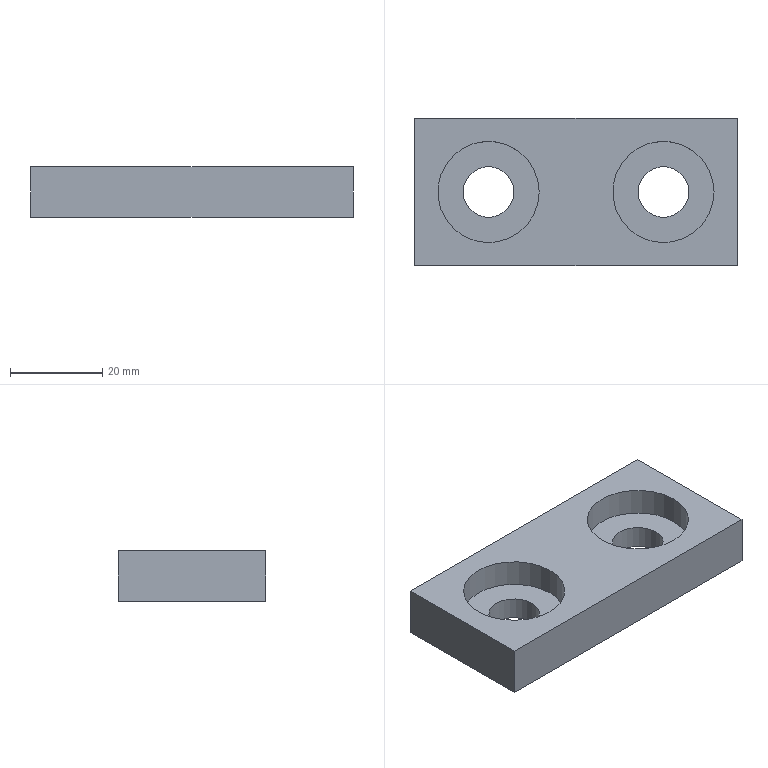Part | NX | features DATUM_CSYS 2, EXTRUDE 2, SKETCH 1 | 1 solid | 12 faces | box 70 x 32 x 11 mm | volume 19128 mm3 | plane 8 | cylinder 4 | commonest cylinder face diameters 11 x2 22 x2
STEP:
#1=CARTESIAN_POINT('',(-35.,16.,0.));
#2=VERTEX_POINT('',#1);
#3=CARTESIAN_POINT('',(-35.,-16.,0.));
#4=VERTEX_POINT('',#3);
#5=CARTESIAN_POINT('',(-35.,16.,0.));
#6=DIRECTION('',(0.,-1.,0.));
#7=VECTOR('',#6,1000.);
#8=LINE('',#5,#7);
#9=EDGE_CURVE('',#2,#4,#8,.T.);
#10=ORIENTED_EDGE('',*,*,#9,.T.);
#11=CARTESIAN_POINT('',(-35.,-16.,11.));
#12=VERTEX_POINT('',#11);
#13=CARTESIAN_POINT('',(-35.,-16.,11.));
#14=DIRECTION('',(0.,0.,-1.));
#15=VECTOR('',#14,1000.);
#16=LINE('',#13,#15);
#17=EDGE_CURVE('',#12,#4,#16,.T.);
#18=ORIENTED_EDGE('',*,*,#17,.F.);
#19=CARTESIAN_POINT('',(-35.,16.,11.));
#20=VERTEX_POINT('',#19);
#21=CARTESIAN_POINT('',(-35.,16.,11.));
#22=DIRECTION('',(0.,-1.,0.));
#23=VECTOR('',#22,1000.);
#24=LINE('',#21,#23);
#25=EDGE_CURVE('',#20,#12,#24,.T.);
#26=ORIENTED_EDGE('',*,*,#25,.F.);
#27=CARTESIAN_POINT('',(-35.,16.,11.));
#28=DIRECTION('',(0.,0.,-1.));
#29=VECTOR('',#28,1000.);
#30=LINE('',#27,#29);
#31=EDGE_CURVE('',#20,#2,#30,.T.);
#32=ORIENTED_EDGE('',*,*,#31,.T.);
#33=EDGE_LOOP('',(#10,#18,#26,#32));
#34=FACE_BOUND('',#33,.T.);
#35=CARTESIAN_POINT('',(-35.,16.,11.));
#36=DIRECTION('',(1.,0.,0.));
#37=DIRECTION('',(0.,0.,-1.));
#38=AXIS2_PLACEMENT_3D('',#35,#36,#37);
#39=PLANE('',#38);
#40=ADVANCED_FACE('',(#34),#39,.F.);
#41=CARTESIAN_POINT('',(35.,-16.,0.));
#42=VERTEX_POINT('',#41);
#43=CARTESIAN_POINT('',(-35.,-16.,0.));
#44=DIRECTION('',(1.,0.,0.));
#45=VECTOR('',#44,1000.);
#46=LINE('',#43,#45);
#47=EDGE_CURVE('',#4,#42,#46,.T.);
#48=ORIENTED_EDGE('',*,*,#47,.T.);
#49=CARTESIAN_POINT('',(35.,-16.,11.));
#50=VERTEX_POINT('',#49);
#51=CARTESIAN_POINT('',(35.,-16.,11.));
#52=DIRECTION('',(0.,0.,-1.));
#53=VECTOR('',#52,1000.);
#54=LINE('',#51,#53);
#55=EDGE_CURVE('',#50,#42,#54,.T.);
#56=ORIENTED_EDGE('',*,*,#55,.F.);
#57=CARTESIAN_POINT('',(-35.,-16.,11.));
#58=DIRECTION('',(1.,0.,0.));
#59=VECTOR('',#58,1000.);
#60=LINE('',#57,#59);
#61=EDGE_CURVE('',#12,#50,#60,.T.);
#62=ORIENTED_EDGE('',*,*,#61,.F.);
#63=ORIENTED_EDGE('',*,*,#17,.T.);
#64=EDGE_LOOP('',(#48,#56,#62,#63));
#65=FACE_BOUND('',#64,.T.);
#66=CARTESIAN_POINT('',(-35.,-16.,11.));
#67=DIRECTION('',(0.,1.,0.));
#68=DIRECTION('',(0.,0.,1.));
#69=AXIS2_PLACEMENT_3D('',#66,#67,#68);
#70=PLANE('',#69);
#71=ADVANCED_FACE('',(#65),#70,.F.);
#72=CARTESIAN_POINT('',(35.,16.,0.));
#73=VERTEX_POINT('',#72);
#74=CARTESIAN_POINT('',(35.,-16.,0.));
#75=DIRECTION('',(0.,1.,0.));
#76=VECTOR('',#75,1000.);
#77=LINE('',#74,#76);
#78=EDGE_CURVE('',#42,#73,#77,.T.);
#79=ORIENTED_EDGE('',*,*,#78,.T.);
#80=CARTESIAN_POINT('',(35.,16.,11.));
#81=VERTEX_POINT('',#80);
#82=CARTESIAN_POINT('',(35.,16.,11.));
#83=DIRECTION('',(0.,0.,-1.));
#84=VECTOR('',#83,1000.);
#85=LINE('',#82,#84);
#86=EDGE_CURVE('',#81,#73,#85,.T.);
#87=ORIENTED_EDGE('',*,*,#86,.F.);
#88=CARTESIAN_POINT('',(35.,-16.,11.));
#89=DIRECTION('',(0.,1.,0.));
#90=VECTOR('',#89,1000.);
#91=LINE('',#88,#90);
#92=EDGE_CURVE('',#50,#81,#91,.T.);
#93=ORIENTED_EDGE('',*,*,#92,.F.);
#94=ORIENTED_EDGE('',*,*,#55,.T.);
#95=EDGE_LOOP('',(#79,#87,#93,#94));
#96=FACE_BOUND('',#95,.T.);
#97=CARTESIAN_POINT('',(35.,-16.,11.));
#98=DIRECTION('',(-1.,0.,0.));
#99=DIRECTION('',(0.,0.,1.));
#100=AXIS2_PLACEMENT_3D('',#97,#98,#99);
#101=PLANE('',#100);
#102=ADVANCED_FACE('',(#96),#101,.F.);
#103=CARTESIAN_POINT('',(-8.,0.,5.));
#104=VERTEX_POINT('',#103);
#105=CARTESIAN_POINT('',(-19.,0.,5.));
#106=DIRECTION('',(0.,0.,1.));
#107=DIRECTION('',(1.,0.,0.));
#108=AXIS2_PLACEMENT_3D('',#105,#106,#107);
#109=CIRCLE('',#108,11.);
#110=EDGE_CURVE('',#104,#104,#109,.T.);
#111=ORIENTED_EDGE('',*,*,#110,.F.);
#112=EDGE_LOOP('',(#111));
#113=FACE_BOUND('',#112,.T.);
#114=CARTESIAN_POINT('',(-8.,0.,11.));
#115=VERTEX_POINT('',#114);
#116=CARTESIAN_POINT('',(-19.,0.,11.));
#117=DIRECTION('',(0.,0.,1.));
#118=DIRECTION('',(1.,0.,0.));
#119=AXIS2_PLACEMENT_3D('',#116,#117,#118);
#120=CIRCLE('',#119,11.);
#121=EDGE_CURVE('',#115,#115,#120,.T.);
#122=ORIENTED_EDGE('',*,*,#121,.T.);
#123=EDGE_LOOP('',(#122));
#124=FACE_BOUND('',#123,.T.);
#125=CARTESIAN_POINT('',(-19.,0.,11.));
#126=DIRECTION('',(0.,0.,-1.));
#127=DIRECTION('',(-1.,0.,0.));
#128=AXIS2_PLACEMENT_3D('',#125,#126,#127);
#129=CYLINDRICAL_SURFACE('',#128,11.);
#130=ADVANCED_FACE('',(#113,#124),#129,.F.);
#131=CARTESIAN_POINT('',(35.,16.,0.));
#132=DIRECTION('',(-1.,0.,0.));
#133=VECTOR('',#132,1000.);
#134=LINE('',#131,#133);
#135=EDGE_CURVE('',#73,#2,#134,.T.);
#136=ORIENTED_EDGE('',*,*,#135,.T.);
#137=ORIENTED_EDGE('',*,*,#31,.F.);
#138=CARTESIAN_POINT('',(35.,16.,11.));
#139=DIRECTION('',(-1.,0.,0.));
#140=VECTOR('',#139,1000.);
#141=LINE('',#138,#140);
#142=EDGE_CURVE('',#81,#20,#141,.T.);
#143=ORIENTED_EDGE('',*,*,#142,.F.);
#144=ORIENTED_EDGE('',*,*,#86,.T.);
#145=EDGE_LOOP('',(#136,#137,#143,#144));
#146=FACE_BOUND('',#145,.T.);
#147=CARTESIAN_POINT('',(35.,16.,11.));
#148=DIRECTION('',(0.,-1.,0.));
#149=DIRECTION('',(0.,0.,-1.));
#150=AXIS2_PLACEMENT_3D('',#147,#148,#149);
#151=PLANE('',#150);
#152=ADVANCED_FACE('',(#146),#151,.F.);
#153=CARTESIAN_POINT('',(30.,0.,5.));
#154=VERTEX_POINT('',#153);
#155=CARTESIAN_POINT('',(19.,0.,5.));
#156=DIRECTION('',(0.,0.,1.));
#157=DIRECTION('',(1.,0.,0.));
#158=AXIS2_PLACEMENT_3D('',#155,#156,#157);
#159=CIRCLE('',#158,11.);
#160=EDGE_CURVE('',#154,#154,#159,.T.);
#161=ORIENTED_EDGE('',*,*,#160,.F.);
#162=EDGE_LOOP('',(#161));
#163=FACE_BOUND('',#162,.T.);
#164=CARTESIAN_POINT('',(30.,0.,11.));
#165=VERTEX_POINT('',#164);
#166=CARTESIAN_POINT('',(19.,0.,11.));
#167=DIRECTION('',(0.,0.,1.));
#168=DIRECTION('',(1.,0.,0.));
#169=AXIS2_PLACEMENT_3D('',#166,#167,#168);
#170=CIRCLE('',#169,11.);
#171=EDGE_CURVE('',#165,#165,#170,.T.);
#172=ORIENTED_EDGE('',*,*,#171,.T.);
#173=EDGE_LOOP('',(#172));
#174=FACE_BOUND('',#173,.T.);
#175=CARTESIAN_POINT('',(19.,0.,11.));
#176=DIRECTION('',(0.,0.,-1.));
#177=DIRECTION('',(-1.,0.,0.));
#178=AXIS2_PLACEMENT_3D('',#175,#176,#177);
#179=CYLINDRICAL_SURFACE('',#178,11.);
#180=ADVANCED_FACE('',(#163,#174),#179,.F.);
#181=ORIENTED_EDGE('',*,*,#25,.T.);
#182=ORIENTED_EDGE('',*,*,#61,.T.);
#183=ORIENTED_EDGE('',*,*,#92,.T.);
#184=ORIENTED_EDGE('',*,*,#142,.T.);
#185=EDGE_LOOP('',(#181,#182,#183,#184));
#186=FACE_BOUND('',#185,.T.);
#187=ORIENTED_EDGE('',*,*,#121,.F.);
#188=EDGE_LOOP('',(#187));
#189=FACE_BOUND('',#188,.T.);
#190=ORIENTED_EDGE('',*,*,#171,.F.);
#191=EDGE_LOOP('',(#190));
#192=FACE_BOUND('',#191,.T.);
#193=CARTESIAN_POINT('',(-19.,0.,11.));
#194=DIRECTION('',(0.,0.,1.));
#195=DIRECTION('',(1.,0.,0.));
#196=AXIS2_PLACEMENT_3D('',#193,#194,#195);
#197=PLANE('',#196);
#198=ADVANCED_FACE('',(#186,#189,#192),#197,.T.);
#199=ORIENTED_EDGE('',*,*,#9,.F.);
#200=ORIENTED_EDGE('',*,*,#135,.F.);
#201=ORIENTED_EDGE('',*,*,#78,.F.);
#202=ORIENTED_EDGE('',*,*,#47,.F.);
#203=EDGE_LOOP('',(#199,#200,#201,#202));
#204=FACE_BOUND('',#203,.T.);
#205=CARTESIAN_POINT('',(24.5,0.,0.));
#206=VERTEX_POINT('',#205);
#207=CARTESIAN_POINT('',(19.,0.,0.));
#208=DIRECTION('',(0.,0.,1.));
#209=DIRECTION('',(1.,0.,0.));
#210=AXIS2_PLACEMENT_3D('',#207,#208,#209);
#211=CIRCLE('',#210,5.5);
#212=EDGE_CURVE('',#206,#206,#211,.T.);
#213=ORIENTED_EDGE('',*,*,#212,.T.);
#214=EDGE_LOOP('',(#213));
#215=FACE_BOUND('',#214,.T.);
#216=CARTESIAN_POINT('',(-13.5,0.,0.));
#217=VERTEX_POINT('',#216);
#218=CARTESIAN_POINT('',(-19.,0.,0.));
#219=DIRECTION('',(0.,0.,1.));
#220=DIRECTION('',(1.,0.,0.));
#221=AXIS2_PLACEMENT_3D('',#218,#219,#220);
#222=CIRCLE('',#221,5.5);
#223=EDGE_CURVE('',#217,#217,#222,.T.);
#224=ORIENTED_EDGE('',*,*,#223,.T.);
#225=EDGE_LOOP('',(#224));
#226=FACE_BOUND('',#225,.T.);
#227=CARTESIAN_POINT('',(-19.,0.,0.));
#228=DIRECTION('',(0.,0.,1.));
#229=DIRECTION('',(1.,0.,0.));
#230=AXIS2_PLACEMENT_3D('',#227,#228,#229);
#231=PLANE('',#230);
#232=ADVANCED_FACE('',(#204,#215,#226),#231,.F.);
#233=CARTESIAN_POINT('',(24.5,0.,5.));
#234=VERTEX_POINT('',#233);
#235=CARTESIAN_POINT('',(19.,0.,5.));
#236=DIRECTION('',(0.,0.,1.));
#237=DIRECTION('',(1.,0.,0.));
#238=AXIS2_PLACEMENT_3D('',#235,#236,#237);
#239=CIRCLE('',#238,5.5);
#240=EDGE_CURVE('',#234,#234,#239,.T.);
#241=ORIENTED_EDGE('',*,*,#240,.T.);
#242=EDGE_LOOP('',(#241));
#243=FACE_BOUND('',#242,.T.);
#244=ORIENTED_EDGE('',*,*,#212,.F.);
#245=EDGE_LOOP('',(#244));
#246=FACE_BOUND('',#245,.T.);
#247=CARTESIAN_POINT('',(19.,0.,5.));
#248=DIRECTION('',(0.,0.,-1.));
#249=DIRECTION('',(-1.,0.,0.));
#250=AXIS2_PLACEMENT_3D('',#247,#248,#249);
#251=CYLINDRICAL_SURFACE('',#250,5.5);
#252=ADVANCED_FACE('',(#243,#246),#251,.F.);
#253=ORIENTED_EDGE('',*,*,#160,.T.);
#254=EDGE_LOOP('',(#253));
#255=FACE_BOUND('',#254,.T.);
#256=ORIENTED_EDGE('',*,*,#240,.F.);
#257=EDGE_LOOP('',(#256));
#258=FACE_BOUND('',#257,.T.);
#259=CARTESIAN_POINT('',(19.,0.,5.));
#260=DIRECTION('',(0.,0.,1.));
#261=DIRECTION('',(1.,0.,0.));
#262=AXIS2_PLACEMENT_3D('',#259,#260,#261);
#263=PLANE('',#262);
#264=ADVANCED_FACE('',(#255,#258),#263,.T.);
#265=CARTESIAN_POINT('',(-13.5,0.,5.));
#266=VERTEX_POINT('',#265);
#267=CARTESIAN_POINT('',(-19.,0.,5.));
#268=DIRECTION('',(0.,0.,1.));
#269=DIRECTION('',(1.,0.,0.));
#270=AXIS2_PLACEMENT_3D('',#267,#268,#269);
#271=CIRCLE('',#270,5.5);
#272=EDGE_CURVE('',#266,#266,#271,.T.);
#273=ORIENTED_EDGE('',*,*,#272,.T.);
#274=EDGE_LOOP('',(#273));
#275=FACE_BOUND('',#274,.T.);
#276=ORIENTED_EDGE('',*,*,#223,.F.);
#277=EDGE_LOOP('',(#276));
#278=FACE_BOUND('',#277,.T.);
#279=CARTESIAN_POINT('',(-19.,0.,5.));
#280=DIRECTION('',(0.,0.,-1.));
#281=DIRECTION('',(-1.,0.,0.));
#282=AXIS2_PLACEMENT_3D('',#279,#280,#281);
#283=CYLINDRICAL_SURFACE('',#282,5.5);
#284=ADVANCED_FACE('',(#275,#278),#283,.F.);
#285=ORIENTED_EDGE('',*,*,#110,.T.);
#286=EDGE_LOOP('',(#285));
#287=FACE_BOUND('',#286,.T.);
#288=ORIENTED_EDGE('',*,*,#272,.F.);
#289=EDGE_LOOP('',(#288));
#290=FACE_BOUND('',#289,.T.);
#291=CARTESIAN_POINT('',(-19.,0.,5.));
#292=DIRECTION('',(0.,0.,1.));
#293=DIRECTION('',(1.,0.,0.));
#294=AXIS2_PLACEMENT_3D('',#291,#292,#293);
#295=PLANE('',#294);
#296=ADVANCED_FACE('',(#287,#290),#295,.T.);
#297=CLOSED_SHELL('',(#40,#71,#102,#130,#152,#180,#198,#232,#252,#264,#284,#296));
#298=MANIFOLD_SOLID_BREP('',#297);
#299=(LENGTH_UNIT()NAMED_UNIT(*)SI_UNIT(.MILLI.,.METRE.));
#300=UNCERTAINTY_MEASURE_WITH_UNIT(LENGTH_MEASURE(0.00001),#299,'','');
#301=(NAMED_UNIT(*)PLANE_ANGLE_UNIT()SI_UNIT($,.RADIAN.));
#302=(NAMED_UNIT(*)SI_UNIT($,.STERADIAN.)SOLID_ANGLE_UNIT());
#303=(GEOMETRIC_REPRESENTATION_CONTEXT(3)GLOBAL_UNCERTAINTY_ASSIGNED_CONTEXT((#300))GLOBAL_UNIT_ASSIGNED_CONTEXT((#299,#301,#302))REPRESENTATION_CONTEXT('',''));
#304=ADVANCED_BREP_SHAPE_REPRESENTATION('',(#298),#303);